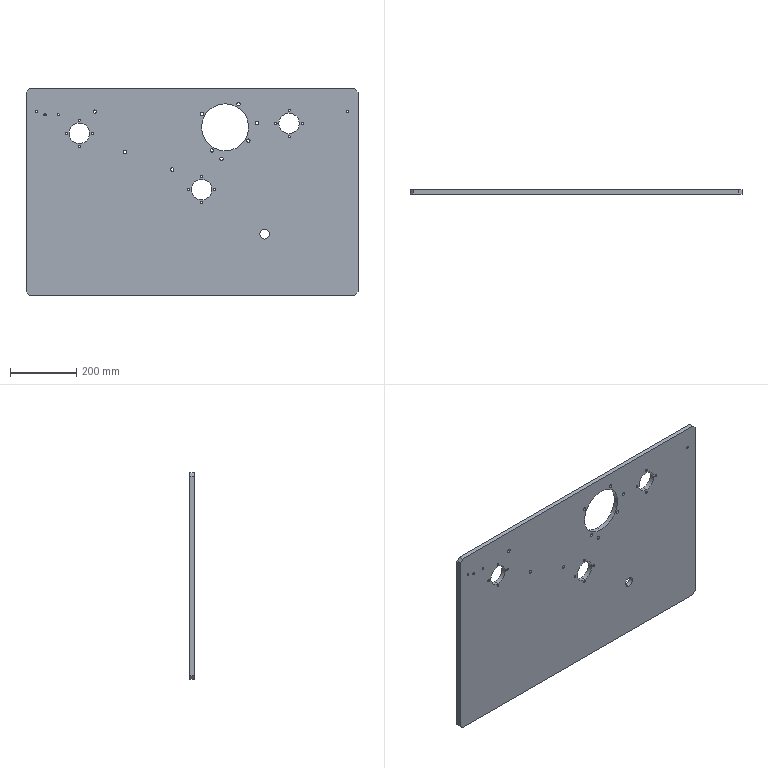Part | SolidWorks | features BaseBody 1 | 1 solid | 70 faces | box 1005 x 14 x 625 mm | volume 8414107 mm3 | cylinder 60 | plane 10 | commonest cylinder face diameters 6.8 x32 10.2 x18 62 x6 30 x2 142 x2